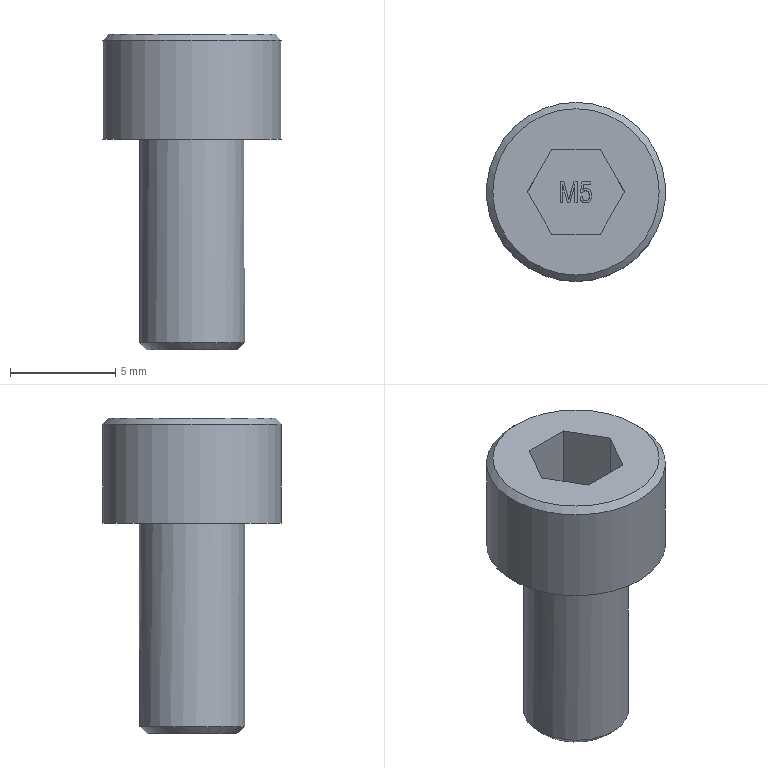Part | STEP file | SOLID | 1 solid | 39 faces | box 8.5 x 8.5 x 15 mm | volume 429.474 mm3 | plane 30 | other 5 | cylinder 2 | cone 2 | commonest cylinder face diameters 5 x1 8.5 x1